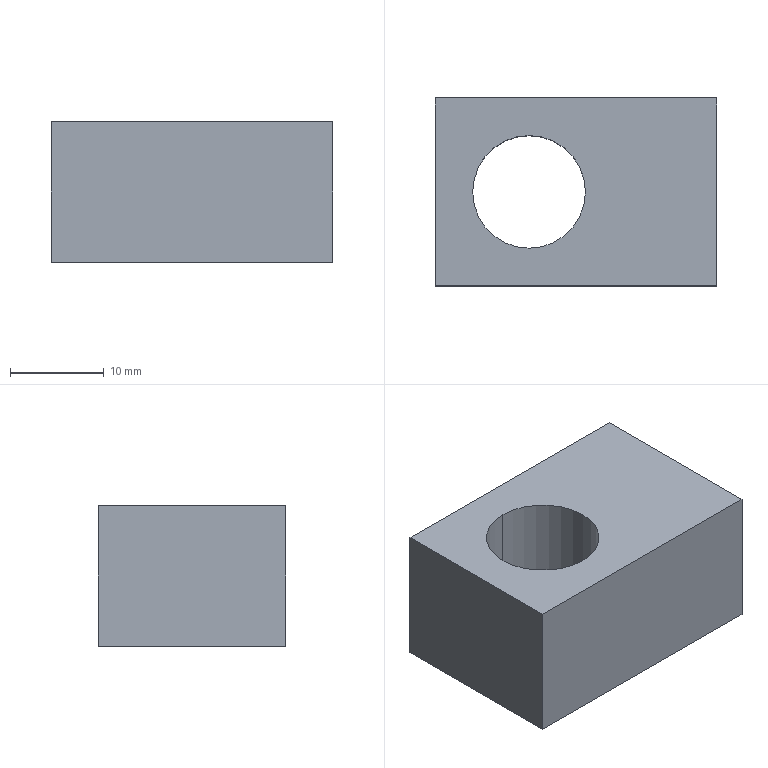Part | STEP file | Positioning_id1962_x_t | 1 solid | 11 faces | box 30 x 20 x 15 mm | volume 7190 mm3 | plane 7 | cylinder 4 | commonest cylinder face diameters 6 x2 12 x2
STEP:
#1=CARTESIAN_POINT('',(0.,0.,0.));
#2=DIRECTION('',(0.,0.,1.));
#3=DIRECTION('',(1.,0.,0.));
#4=AXIS2_PLACEMENT_3D('',#1,#2,#3);
#5=CARTESIAN_POINT('',(-706.002,0.5,354.5));
#6=VERTEX_POINT('',#5);
#7=CARTESIAN_POINT('',(-706.002,-5.5,354.5));
#8=VERTEX_POINT('',#7);
#9=CARTESIAN_POINT('',(-706.002,-2.5,354.5));
#10=DIRECTION('',(-1.,0.,0.));
#11=DIRECTION('',(0.,0.,-1.));
#12=AXIS2_PLACEMENT_3D('',#9,#10,#11);
#13=CIRCLE('',#12,3.);
#14=CARTESIAN_POINT('',(-656.002,-2.5,354.5));
#15=DIRECTION('',(1.,0.,0.));
#16=DIRECTION('',(0.,-1.,0.));
#17=AXIS2_PLACEMENT_3D('',#14,#15,#16);
#18=CYLINDRICAL_SURFACE('',#17,3.);
#19=CARTESIAN_POINT('',(7.854,-50.));
#20=DIRECTION('',(-1.,0.));
#21=VECTOR('',#20,1.);
#22=LINE('',#19,#21);
#23=(GEOMETRIC_REPRESENTATION_CONTEXT(2)PARAMETRIC_REPRESENTATION_CONTEXT()REPRESENTATION_CONTEXT('',''));
#24=DEFINITIONAL_REPRESENTATION('',(#22),#23);
#25=PCURVE('',#18,#24);
#26=CARTESIAN_POINT('',(-706.002,-2.5,354.5));
#27=DIRECTION('',(-1.,0.,0.));
#28=DIRECTION('',(0.,-1.,0.));
#29=AXIS2_PLACEMENT_3D('',#26,#27,#28);
#30=PLANE('',#29);
#31=CARTESIAN_POINT('',(0.,0.));
#32=DIRECTION('',(0.,-1.));
#33=AXIS2_PLACEMENT_2D('',#31,#32);
#34=CIRCLE('',#33,3.);
#35=(GEOMETRIC_REPRESENTATION_CONTEXT(2)PARAMETRIC_REPRESENTATION_CONTEXT()REPRESENTATION_CONTEXT('',''));
#36=DEFINITIONAL_REPRESENTATION('',(#34),#35);
#37=PCURVE('',#30,#36);
#38=SURFACE_CURVE('',#13,(#25,#37),.PCURVE_S1.);
#39=EDGE_CURVE('',#6,#8,#38,.T.);
#40=ORIENTED_EDGE('',*,*,#39,.F.);
#41=CARTESIAN_POINT('',(-702.002,0.5,354.5));
#42=VERTEX_POINT('',#41);
#43=CARTESIAN_POINT('',(-702.002,0.5,354.5));
#44=DIRECTION('',(1.,0.,0.));
#45=VECTOR('',#44,1.);
#46=LINE('',#43,#45);
#47=CARTESIAN_POINT('',(3.142,-46.));
#48=DIRECTION('',(0.,1.));
#49=VECTOR('',#48,1.);
#50=LINE('',#47,#49);
#51=(GEOMETRIC_REPRESENTATION_CONTEXT(2)PARAMETRIC_REPRESENTATION_CONTEXT()REPRESENTATION_CONTEXT('',''));
#52=DEFINITIONAL_REPRESENTATION('',(#50),#51);
#53=PCURVE('',#18,#52);
#54=CARTESIAN_POINT('',(-656.002,-2.5,354.5));
#55=DIRECTION('',(1.,0.,0.));
#56=DIRECTION('',(0.,-1.,0.));
#57=AXIS2_PLACEMENT_3D('',#54,#55,#56);
#58=CYLINDRICAL_SURFACE('',#57,3.);
#59=CARTESIAN_POINT('',(3.142,-46.));
#60=DIRECTION('',(0.,1.));
#61=VECTOR('',#60,1.);
#62=LINE('',#59,#61);
#63=(GEOMETRIC_REPRESENTATION_CONTEXT(2)PARAMETRIC_REPRESENTATION_CONTEXT()REPRESENTATION_CONTEXT('',''));
#64=DEFINITIONAL_REPRESENTATION('',(#62),#63);
#65=PCURVE('',#58,#64);
#66=SURFACE_CURVE('',#46,(#53,#65),.PCURVE_S1.);
#67=EDGE_CURVE('',#6,#42,#66,.T.);
#68=ORIENTED_EDGE('',*,*,#67,.T.);
#69=CARTESIAN_POINT('',(-702.002,-5.5,354.5));
#70=VERTEX_POINT('',#69);
#71=CARTESIAN_POINT('',(-702.002,-2.5,354.5));
#72=DIRECTION('',(1.,0.,0.));
#73=DIRECTION('',(0.,0.,-1.));
#74=AXIS2_PLACEMENT_3D('',#71,#72,#73);
#75=CIRCLE('',#74,3.);
#76=CARTESIAN_POINT('',(-4.712,-46.));
#77=DIRECTION('',(1.,0.));
#78=VECTOR('',#77,1.);
#79=LINE('',#76,#78);
#80=(GEOMETRIC_REPRESENTATION_CONTEXT(2)PARAMETRIC_REPRESENTATION_CONTEXT()REPRESENTATION_CONTEXT('',''));
#81=DEFINITIONAL_REPRESENTATION('',(#79),#80);
#82=PCURVE('',#18,#81);
#83=CARTESIAN_POINT('',(-702.002,12.5,362.));
#84=DIRECTION('',(1.,0.,0.));
#85=DIRECTION('',(0.,-1.,0.));
#86=AXIS2_PLACEMENT_3D('',#83,#84,#85);
#87=PLANE('',#86);
#88=CARTESIAN_POINT('',(15.,7.5));
#89=DIRECTION('',(0.,1.));
#90=AXIS2_PLACEMENT_2D('',#88,#89);
#91=CIRCLE('',#90,3.);
#92=(GEOMETRIC_REPRESENTATION_CONTEXT(2)PARAMETRIC_REPRESENTATION_CONTEXT()REPRESENTATION_CONTEXT('',''));
#93=DEFINITIONAL_REPRESENTATION('',(#91),#92);
#94=PCURVE('',#87,#93);
#95=SURFACE_CURVE('',#75,(#82,#94),.PCURVE_S1.);
#96=EDGE_CURVE('',#70,#42,#95,.T.);
#97=ORIENTED_EDGE('',*,*,#96,.F.);
#98=CARTESIAN_POINT('',(-702.002,-5.5,354.5));
#99=DIRECTION('',(-1.,0.,0.));
#100=VECTOR('',#99,1.);
#101=LINE('',#98,#100);
#102=CARTESIAN_POINT('',(0.,-46.));
#103=DIRECTION('',(0.,-1.));
#104=VECTOR('',#103,1.);
#105=LINE('',#102,#104);
#106=(GEOMETRIC_REPRESENTATION_CONTEXT(2)PARAMETRIC_REPRESENTATION_CONTEXT()REPRESENTATION_CONTEXT('',''));
#107=DEFINITIONAL_REPRESENTATION('',(#105),#106);
#108=PCURVE('',#18,#107);
#109=CARTESIAN_POINT('',(6.283,-46.));
#110=DIRECTION('',(0.,-1.));
#111=VECTOR('',#110,1.);
#112=LINE('',#109,#111);
#113=(GEOMETRIC_REPRESENTATION_CONTEXT(2)PARAMETRIC_REPRESENTATION_CONTEXT()REPRESENTATION_CONTEXT('',''));
#114=DEFINITIONAL_REPRESENTATION('',(#112),#113);
#115=PCURVE('',#58,#114);
#116=SURFACE_CURVE('',#101,(#108,#115),.PCURVE_S1.);
#117=EDGE_CURVE('',#70,#8,#116,.T.);
#118=ORIENTED_EDGE('',*,*,#117,.T.);
#119=EDGE_LOOP('',(#40,#68,#97,#118));
#120=FACE_BOUND('',#119,.F.);
#121=ADVANCED_FACE('',(#120),#18,.F.);
#122=ORIENTED_EDGE('',*,*,#39,.F.);
#123=CARTESIAN_POINT('',(-706.002,-5.5,354.5));
#124=CARTESIAN_POINT('',(-706.002,-5.5,357.5));
#125=CARTESIAN_POINT('',(-706.002,-2.5,359.));
#126=CARTESIAN_POINT('',(-706.002,0.5,357.5));
#127=CARTESIAN_POINT('',(-706.002,0.5,354.5));
#128=(BOUNDED_CURVE()B_SPLINE_CURVE(4,(#123,#124,#125,#126,#127),.UNSPECIFIED.,.F.,.F.)B_SPLINE_CURVE_WITH_KNOTS((5,5),(0.,1.),.PIECEWISE_BEZIER_KNOTS.)CURVE()GEOMETRIC_REPRESENTATION_ITEM()RATIONAL_B_SPLINE_CURVE((1.,0.7071,0.6667,0.7071,1.))REPRESENTATION_ITEM(''));
#129=CARTESIAN_POINT('',(3.,0.));
#130=CARTESIAN_POINT('',(3.,3.));
#131=CARTESIAN_POINT('',(0.,4.5));
#132=CARTESIAN_POINT('',(-3.,3.));
#133=CARTESIAN_POINT('',(-3.,0.));
#134=(BOUNDED_CURVE()B_SPLINE_CURVE(4,(#129,#130,#131,#132,#133),.UNSPECIFIED.,.F.,.F.)B_SPLINE_CURVE_WITH_KNOTS((5,5),(0.,1.),.PIECEWISE_BEZIER_KNOTS.)CURVE()GEOMETRIC_REPRESENTATION_ITEM()RATIONAL_B_SPLINE_CURVE((1.,0.7071,0.6667,0.7071,1.))REPRESENTATION_ITEM(''));
#135=(GEOMETRIC_REPRESENTATION_CONTEXT(2)PARAMETRIC_REPRESENTATION_CONTEXT()REPRESENTATION_CONTEXT('',''));
#136=DEFINITIONAL_REPRESENTATION('',(#134),#135);
#137=PCURVE('',#30,#136);
#138=CARTESIAN_POINT('',(6.283,-50.));
#139=CARTESIAN_POINT('',(6.24,-50.));
#140=CARTESIAN_POINT('',(6.153,-50.));
#141=CARTESIAN_POINT('',(6.02,-50.));
#142=CARTESIAN_POINT('',(5.883,-50.));
#143=CARTESIAN_POINT('',(5.744,-50.));
#144=CARTESIAN_POINT('',(5.602,-50.));
#145=CARTESIAN_POINT('',(5.457,-50.));
#146=CARTESIAN_POINT('',(5.311,-50.));
#147=CARTESIAN_POINT('',(5.163,-50.));
#148=CARTESIAN_POINT('',(5.013,-50.));
#149=CARTESIAN_POINT('',(4.863,-50.));
#150=CARTESIAN_POINT('',(4.712,-50.));
#151=CARTESIAN_POINT('',(4.562,-50.));
#152=CARTESIAN_POINT('',(4.412,-50.));
#153=CARTESIAN_POINT('',(4.262,-50.));
#154=CARTESIAN_POINT('',(4.114,-50.));
#155=CARTESIAN_POINT('',(3.968,-50.));
#156=CARTESIAN_POINT('',(3.823,-50.));
#157=CARTESIAN_POINT('',(3.681,-50.));
#158=CARTESIAN_POINT('',(3.542,-50.));
#159=CARTESIAN_POINT('',(3.405,-50.));
#160=CARTESIAN_POINT('',(3.271,-50.));
#161=CARTESIAN_POINT('',(3.184,-50.));
#162=CARTESIAN_POINT('',(3.142,-50.));
#163=B_SPLINE_CURVE_WITH_KNOTS('',3,(#138,#139,#140,#141,#142,#143,#144,#145,#146,#147,#148,#149,#150,#151,#152,#153,#154,#155,#156,#157,#158,#159,#160,#161,#162),.UNSPECIFIED.,.F.,.F.,(4,1,1,1,1,1,1,1,1,1,1,1,1,1,1,1,1,1,1,1,1,1,4),(0.,0.04545,0.09091,0.1364,0.1818,0.2273,0.2727,0.3182,0.3636,0.4091,0.4545,0.5,0.5455,0.5909,0.6364,0.6818,0.7273,0.7727,0.8182,0.8636,0.9091,0.9545,1.),.QUASI_UNIFORM_KNOTS.);
#164=(GEOMETRIC_REPRESENTATION_CONTEXT(2)PARAMETRIC_REPRESENTATION_CONTEXT()REPRESENTATION_CONTEXT('',''));
#165=DEFINITIONAL_REPRESENTATION('',(#163),#164);
#166=PCURVE('',#58,#165);
#167=SURFACE_CURVE('',#128,(#137,#166),.PCURVE_S1.);
#168=EDGE_CURVE('',#8,#6,#167,.T.);
#169=ORIENTED_EDGE('',*,*,#168,.F.);
#170=EDGE_LOOP('',(#122,#169));
#171=FACE_BOUND('',#170,.T.);
#172=ADVANCED_FACE('',(#171),#30,.F.);
#173=CARTESIAN_POINT('',(-702.002,-10.,362.));
#174=VERTEX_POINT('',#173);
#175=CARTESIAN_POINT('',(-732.002,-10.,362.));
#176=VERTEX_POINT('',#175);
#177=CARTESIAN_POINT('',(-702.002,-10.,362.));
#178=DIRECTION('',(-1.,0.,0.));
#179=VECTOR('',#178,1.);
#180=LINE('',#177,#179);
#181=CARTESIAN_POINT('',(-656.002,-10.,364.5));
#182=DIRECTION('',(0.,-1.,0.));
#183=DIRECTION('',(0.,0.,1.));
#184=AXIS2_PLACEMENT_3D('',#181,#182,#183);
#185=PLANE('',#184);
#186=CARTESIAN_POINT('',(-2.5,46.));
#187=DIRECTION('',(0.,1.));
#188=VECTOR('',#187,1.);
#189=LINE('',#186,#188);
#190=(GEOMETRIC_REPRESENTATION_CONTEXT(2)PARAMETRIC_REPRESENTATION_CONTEXT()REPRESENTATION_CONTEXT('',''));
#191=DEFINITIONAL_REPRESENTATION('',(#189),#190);
#192=PCURVE('',#185,#191);
#193=CARTESIAN_POINT('',(-714.502,-6.25,362.));
#194=DIRECTION('',(0.,0.,1.));
#195=DIRECTION('',(1.,0.,0.));
#196=AXIS2_PLACEMENT_3D('',#193,#194,#195);
#197=PLANE('',#196);
#198=CARTESIAN_POINT('',(12.5,-3.75));
#199=DIRECTION('',(-1.,0.));
#200=VECTOR('',#199,1.);
#201=LINE('',#198,#200);
#202=(GEOMETRIC_REPRESENTATION_CONTEXT(2)PARAMETRIC_REPRESENTATION_CONTEXT()REPRESENTATION_CONTEXT('',''));
#203=DEFINITIONAL_REPRESENTATION('',(#201),#202);
#204=PCURVE('',#197,#203);
#205=SURFACE_CURVE('',#180,(#192,#204),.PCURVE_S1.);
#206=EDGE_CURVE('',#174,#176,#205,.T.);
#207=ORIENTED_EDGE('',*,*,#206,.T.);
#208=CARTESIAN_POINT('',(-732.002,-10.,347.));
#209=VERTEX_POINT('',#208);
#210=CARTESIAN_POINT('',(-732.002,-10.,362.));
#211=DIRECTION('',(0.,0.,-1.));
#212=VECTOR('',#211,1.);
#213=LINE('',#210,#212);
#214=CARTESIAN_POINT('',(-2.5,76.));
#215=DIRECTION('',(-1.,0.));
#216=VECTOR('',#215,1.);
#217=LINE('',#214,#216);
#218=(GEOMETRIC_REPRESENTATION_CONTEXT(2)PARAMETRIC_REPRESENTATION_CONTEXT()REPRESENTATION_CONTEXT('',''));
#219=DEFINITIONAL_REPRESENTATION('',(#217),#218);
#220=PCURVE('',#185,#219);
#221=CARTESIAN_POINT('',(-732.002,-6.25,354.5));
#222=DIRECTION('',(-1.,0.,0.));
#223=DIRECTION('',(0.,0.,1.));
#224=AXIS2_PLACEMENT_3D('',#221,#222,#223);
#225=PLANE('',#224);
#226=CARTESIAN_POINT('',(7.5,-3.75));
#227=DIRECTION('',(-1.,0.));
#228=VECTOR('',#227,1.);
#229=LINE('',#226,#228);
#230=(GEOMETRIC_REPRESENTATION_CONTEXT(2)PARAMETRIC_REPRESENTATION_CONTEXT()REPRESENTATION_CONTEXT('',''));
#231=DEFINITIONAL_REPRESENTATION('',(#229),#230);
#232=PCURVE('',#225,#231);
#233=SURFACE_CURVE('',#213,(#220,#232),.PCURVE_S1.);
#234=EDGE_CURVE('',#176,#209,#233,.T.);
#235=ORIENTED_EDGE('',*,*,#234,.T.);
#236=CARTESIAN_POINT('',(-702.002,-10.,347.));
#237=VERTEX_POINT('',#236);
#238=CARTESIAN_POINT('',(-732.002,-10.,347.));
#239=DIRECTION('',(1.,0.,0.));
#240=VECTOR('',#239,1.);
#241=LINE('',#238,#240);
#242=CARTESIAN_POINT('',(-17.5,76.));
#243=DIRECTION('',(0.,-1.));
#244=VECTOR('',#243,1.);
#245=LINE('',#242,#244);
#246=(GEOMETRIC_REPRESENTATION_CONTEXT(2)PARAMETRIC_REPRESENTATION_CONTEXT()REPRESENTATION_CONTEXT('',''));
#247=DEFINITIONAL_REPRESENTATION('',(#245),#246);
#248=PCURVE('',#185,#247);
#249=CARTESIAN_POINT('',(-714.502,-6.25,347.));
#250=DIRECTION('',(0.,0.,-1.));
#251=DIRECTION('',(-1.,0.,0.));
#252=AXIS2_PLACEMENT_3D('',#249,#250,#251);
#253=PLANE('',#252);
#254=CARTESIAN_POINT('',(17.5,-3.75));
#255=DIRECTION('',(-1.,0.));
#256=VECTOR('',#255,1.);
#257=LINE('',#254,#256);
#258=(GEOMETRIC_REPRESENTATION_CONTEXT(2)PARAMETRIC_REPRESENTATION_CONTEXT()REPRESENTATION_CONTEXT('',''));
#259=DEFINITIONAL_REPRESENTATION('',(#257),#258);
#260=PCURVE('',#253,#259);
#261=SURFACE_CURVE('',#241,(#248,#260),.PCURVE_S1.);
#262=EDGE_CURVE('',#209,#237,#261,.T.);
#263=ORIENTED_EDGE('',*,*,#262,.T.);
#264=CARTESIAN_POINT('',(-702.002,-10.,362.));
#265=DIRECTION('',(0.,0.,-1.));
#266=VECTOR('',#265,1.);
#267=LINE('',#264,#266);
#268=CARTESIAN_POINT('',(-2.5,46.));
#269=DIRECTION('',(-1.,0.));
#270=VECTOR('',#269,1.);
#271=LINE('',#268,#270);
#272=(GEOMETRIC_REPRESENTATION_CONTEXT(2)PARAMETRIC_REPRESENTATION_CONTEXT()REPRESENTATION_CONTEXT('',''));
#273=DEFINITIONAL_REPRESENTATION('',(#271),#272);
#274=PCURVE('',#185,#273);
#275=CARTESIAN_POINT('',(22.5,0.));
#276=DIRECTION('',(0.,1.));
#277=VECTOR('',#276,1.);
#278=LINE('',#275,#277);
#279=(GEOMETRIC_REPRESENTATION_CONTEXT(2)PARAMETRIC_REPRESENTATION_CONTEXT()REPRESENTATION_CONTEXT('',''));
#280=DEFINITIONAL_REPRESENTATION('',(#278),#279);
#281=PCURVE('',#87,#280);
#282=SURFACE_CURVE('',#267,(#274,#281),.PCURVE_S1.);
#283=EDGE_CURVE('',#174,#237,#282,.T.);
#284=ORIENTED_EDGE('',*,*,#283,.F.);
#285=EDGE_LOOP('',(#207,#235,#263,#284));
#286=FACE_BOUND('',#285,.T.);
#287=ADVANCED_FACE('',(#286),#185,.T.);
#288=CARTESIAN_POINT('',(-722.002,-6.,347.));
#289=VERTEX_POINT('',#288);
#290=CARTESIAN_POINT('',(-722.002,6.,347.));
#291=VERTEX_POINT('',#290);
#292=CARTESIAN_POINT('',(-722.002,-0.00002593,347.));
#293=DIRECTION('',(0.,0.,-1.));
#294=DIRECTION('',(0.,-1.,0.));
#295=AXIS2_PLACEMENT_3D('',#292,#293,#294);
#296=CIRCLE('',#295,6.);
#297=CARTESIAN_POINT('',(7.5,6.25));
#298=DIRECTION('',(0.,-1.));
#299=AXIS2_PLACEMENT_2D('',#297,#298);
#300=CIRCLE('',#299,6.);
#301=(GEOMETRIC_REPRESENTATION_CONTEXT(2)PARAMETRIC_REPRESENTATION_CONTEXT()REPRESENTATION_CONTEXT('',''));
#302=DEFINITIONAL_REPRESENTATION('',(#300),#301);
#303=PCURVE('',#253,#302);
#304=CARTESIAN_POINT('',(-722.002,-0.00002593,342.));
#305=DIRECTION('',(0.,0.,-1.));
#306=DIRECTION('',(0.,1.,0.));
#307=AXIS2_PLACEMENT_3D('',#304,#305,#306);
#308=CYLINDRICAL_SURFACE('',#307,6.);
#309=CARTESIAN_POINT('',(3.142,-5.));
#310=DIRECTION('',(1.,0.));
#311=VECTOR('',#310,1.);
#312=LINE('',#309,#311);
#313=(GEOMETRIC_REPRESENTATION_CONTEXT(2)PARAMETRIC_REPRESENTATION_CONTEXT()REPRESENTATION_CONTEXT('',''));
#314=DEFINITIONAL_REPRESENTATION('',(#312),#313);
#315=PCURVE('',#308,#314);
#316=SURFACE_CURVE('',#296,(#303,#315),.PCURVE_S1.);
#317=EDGE_CURVE('',#289,#291,#316,.T.);
#318=ORIENTED_EDGE('',*,*,#317,.F.);
#319=CARTESIAN_POINT('',(-722.002,-0.00002593,347.));
#320=DIRECTION('',(0.,0.,-1.));
#321=DIRECTION('',(0.,1.,0.));
#322=AXIS2_PLACEMENT_3D('',#319,#320,#321);
#323=CIRCLE('',#322,6.);
#324=CARTESIAN_POINT('',(7.5,6.25));
#325=DIRECTION('',(0.,1.));
#326=AXIS2_PLACEMENT_2D('',#324,#325);
#327=CIRCLE('',#326,6.);
#328=(GEOMETRIC_REPRESENTATION_CONTEXT(2)PARAMETRIC_REPRESENTATION_CONTEXT()REPRESENTATION_CONTEXT('',''));
#329=DEFINITIONAL_REPRESENTATION('',(#327),#328);
#330=PCURVE('',#253,#329);
#331=CARTESIAN_POINT('',(-722.002,-0.00002593,342.));
#332=DIRECTION('',(0.,0.,-1.));
#333=DIRECTION('',(0.,1.,0.));
#334=AXIS2_PLACEMENT_3D('',#331,#332,#333);
#335=CYLINDRICAL_SURFACE('',#334,6.);
#336=CARTESIAN_POINT('',(0.,-5.));
#337=DIRECTION('',(1.,0.));
#338=VECTOR('',#337,1.);
#339=LINE('',#336,#338);
#340=(GEOMETRIC_REPRESENTATION_CONTEXT(2)PARAMETRIC_REPRESENTATION_CONTEXT()REPRESENTATION_CONTEXT('',''));
#341=DEFINITIONAL_REPRESENTATION('',(#339),#340);
#342=PCURVE('',#335,#341);
#343=SURFACE_CURVE('',#323,(#330,#342),.PCURVE_S1.);
#344=EDGE_CURVE('',#291,#289,#343,.T.);
#345=ORIENTED_EDGE('',*,*,#344,.F.);
#346=EDGE_LOOP('',(#318,#345));
#347=FACE_BOUND('',#346,.T.);
#348=CARTESIAN_POINT('',(-702.002,10.,347.));
#349=VERTEX_POINT('',#348);
#350=CARTESIAN_POINT('',(-732.002,10.,347.));
#351=VERTEX_POINT('',#350);
#352=CARTESIAN_POINT('',(-702.002,10.,347.));
#353=DIRECTION('',(-1.,0.,0.));
#354=VECTOR('',#353,1.);
#355=LINE('',#352,#354);
#356=CARTESIAN_POINT('',(-12.5,16.25));
#357=DIRECTION('',(1.,0.));
#358=VECTOR('',#357,1.);
#359=LINE('',#356,#358);
#360=(GEOMETRIC_REPRESENTATION_CONTEXT(2)PARAMETRIC_REPRESENTATION_CONTEXT()REPRESENTATION_CONTEXT('',''));
#361=DEFINITIONAL_REPRESENTATION('',(#359),#360);
#362=PCURVE('',#253,#361);
#363=CARTESIAN_POINT('',(-714.502,10.,354.5));
#364=DIRECTION('',(0.,1.,0.));
#365=DIRECTION('',(0.,0.,-1.));
#366=AXIS2_PLACEMENT_3D('',#363,#364,#365);
#367=PLANE('',#366);
#368=CARTESIAN_POINT('',(7.5,-12.5));
#369=DIRECTION('',(0.,1.));
#370=VECTOR('',#369,1.);
#371=LINE('',#368,#370);
#372=(GEOMETRIC_REPRESENTATION_CONTEXT(2)PARAMETRIC_REPRESENTATION_CONTEXT()REPRESENTATION_CONTEXT('',''));
#373=DEFINITIONAL_REPRESENTATION('',(#371),#372);
#374=PCURVE('',#367,#373);
#375=SURFACE_CURVE('',#355,(#362,#374),.PCURVE_S1.);
#376=EDGE_CURVE('',#349,#351,#375,.T.);
#377=ORIENTED_EDGE('',*,*,#376,.F.);
#378=CARTESIAN_POINT('',(-702.002,-10.,347.));
#379=DIRECTION('',(0.,1.,0.));
#380=VECTOR('',#379,1.);
#381=LINE('',#378,#380);
#382=CARTESIAN_POINT('',(-12.5,-3.75));
#383=DIRECTION('',(0.,1.));
#384=VECTOR('',#383,1.);
#385=LINE('',#382,#384);
#386=(GEOMETRIC_REPRESENTATION_CONTEXT(2)PARAMETRIC_REPRESENTATION_CONTEXT()REPRESENTATION_CONTEXT('',''));
#387=DEFINITIONAL_REPRESENTATION('',(#385),#386);
#388=PCURVE('',#253,#387);
#389=CARTESIAN_POINT('',(22.5,15.));
#390=DIRECTION('',(-1.,0.));
#391=VECTOR('',#390,1.);
#392=LINE('',#389,#391);
#393=(GEOMETRIC_REPRESENTATION_CONTEXT(2)PARAMETRIC_REPRESENTATION_CONTEXT()REPRESENTATION_CONTEXT('',''));
#394=DEFINITIONAL_REPRESENTATION('',(#392),#393);
#395=PCURVE('',#87,#394);
#396=SURFACE_CURVE('',#381,(#388,#395),.PCURVE_S1.);
#397=EDGE_CURVE('',#237,#349,#396,.T.);
#398=ORIENTED_EDGE('',*,*,#397,.F.);
#399=ORIENTED_EDGE('',*,*,#262,.F.);
#400=CARTESIAN_POINT('',(-732.002,10.,347.));
#401=DIRECTION('',(0.,-1.,0.));
#402=VECTOR('',#401,1.);
#403=LINE('',#400,#402);
#404=CARTESIAN_POINT('',(17.5,16.25));
#405=DIRECTION('',(0.,-1.));
#406=VECTOR('',#405,1.);
#407=LINE('',#404,#406);
#408=(GEOMETRIC_REPRESENTATION_CONTEXT(2)PARAMETRIC_REPRESENTATION_CONTEXT()REPRESENTATION_CONTEXT('',''));
#409=DEFINITIONAL_REPRESENTATION('',(#407),#408);
#410=PCURVE('',#253,#409);
#411=CARTESIAN_POINT('',(-7.5,16.25));
#412=DIRECTION('',(0.,-1.));
#413=VECTOR('',#412,1.);
#414=LINE('',#411,#413);
#415=(GEOMETRIC_REPRESENTATION_CONTEXT(2)PARAMETRIC_REPRESENTATION_CONTEXT()REPRESENTATION_CONTEXT('',''));
#416=DEFINITIONAL_REPRESENTATION('',(#414),#415);
#417=PCURVE('',#225,#416);
#418=SURFACE_CURVE('',#403,(#410,#417),.PCURVE_S1.);
#419=EDGE_CURVE('',#351,#209,#418,.T.);
#420=ORIENTED_EDGE('',*,*,#419,.F.);
#421=EDGE_LOOP('',(#377,#398,#399,#420));
#422=FACE_BOUND('',#421,.T.);
#423=ADVANCED_FACE('',(#347,#422),#253,.T.);
#424=CARTESIAN_POINT('',(-702.002,10.,362.));
#425=VERTEX_POINT('',#424);
#426=CARTESIAN_POINT('',(-702.002,10.,362.));
#427=DIRECTION('',(0.,0.,-1.));
#428=VECTOR('',#427,1.);
#429=LINE('',#426,#428);
#430=CARTESIAN_POINT('',(-7.5,-12.5));
#431=DIRECTION('',(1.,0.));
#432=VECTOR('',#431,1.);
#433=LINE('',#430,#432);
#434=(GEOMETRIC_REPRESENTATION_CONTEXT(2)PARAMETRIC_REPRESENTATION_CONTEXT()REPRESENTATION_CONTEXT('',''));
#435=DEFINITIONAL_REPRESENTATION('',(#433),#434);
#436=PCURVE('',#367,#435);
#437=CARTESIAN_POINT('',(2.5,0.));
#438=DIRECTION('',(0.,1.));
#439=VECTOR('',#438,1.);
#440=LINE('',#437,#439);
#441=(GEOMETRIC_REPRESENTATION_CONTEXT(2)PARAMETRIC_REPRESENTATION_CONTEXT()REPRESENTATION_CONTEXT('',''));
#442=DEFINITIONAL_REPRESENTATION('',(#440),#441);
#443=PCURVE('',#87,#442);
#444=SURFACE_CURVE('',#429,(#436,#443),.PCURVE_S1.);
#445=EDGE_CURVE('',#425,#349,#444,.T.);
#446=ORIENTED_EDGE('',*,*,#445,.T.);
#447=ORIENTED_EDGE('',*,*,#376,.T.);
#448=CARTESIAN_POINT('',(-732.002,10.,362.));
#449=VERTEX_POINT('',#448);
#450=CARTESIAN_POINT('',(-732.002,10.,362.));
#451=DIRECTION('',(0.,0.,-1.));
#452=VECTOR('',#451,1.);
#453=LINE('',#450,#452);
#454=CARTESIAN_POINT('',(-7.5,17.5));
#455=DIRECTION('',(1.,0.));
#456=VECTOR('',#455,1.);
#457=LINE('',#454,#456);
#458=(GEOMETRIC_REPRESENTATION_CONTEXT(2)PARAMETRIC_REPRESENTATION_CONTEXT()REPRESENTATION_CONTEXT('',''));
#459=DEFINITIONAL_REPRESENTATION('',(#457),#458);
#460=PCURVE('',#367,#459);
#461=CARTESIAN_POINT('',(7.5,16.25));
#462=DIRECTION('',(-1.,0.));
#463=VECTOR('',#462,1.);
#464=LINE('',#461,#463);
#465=(GEOMETRIC_REPRESENTATION_CONTEXT(2)PARAMETRIC_REPRESENTATION_CONTEXT()REPRESENTATION_CONTEXT('',''));
#466=DEFINITIONAL_REPRESENTATION('',(#464),#465);
#467=PCURVE('',#225,#466);
#468=SURFACE_CURVE('',#453,(#460,#467),.PCURVE_S1.);
#469=EDGE_CURVE('',#449,#351,#468,.T.);
#470=ORIENTED_EDGE('',*,*,#469,.F.);
#471=CARTESIAN_POINT('',(-732.002,10.,362.));
#472=DIRECTION('',(1.,0.,0.));
#473=VECTOR('',#472,1.);
#474=LINE('',#471,#473);
#475=CARTESIAN_POINT('',(-7.5,17.5));
#476=DIRECTION('',(0.,-1.));
#477=VECTOR('',#476,1.);
#478=LINE('',#475,#477);
#479=(GEOMETRIC_REPRESENTATION_CONTEXT(2)PARAMETRIC_REPRESENTATION_CONTEXT()REPRESENTATION_CONTEXT('',''));
#480=DEFINITIONAL_REPRESENTATION('',(#478),#479);
#481=PCURVE('',#367,#480);
#482=CARTESIAN_POINT('',(-17.5,16.25));
#483=DIRECTION('',(1.,0.));
#484=VECTOR('',#483,1.);
#485=LINE('',#482,#484);
#486=(GEOMETRIC_REPRESENTATION_CONTEXT(2)PARAMETRIC_REPRESENTATION_CONTEXT()REPRESENTATION_CONTEXT('',''));
#487=DEFINITIONAL_REPRESENTATION('',(#485),#486);
#488=PCURVE('',#197,#487);
#489=SURFACE_CURVE('',#474,(#481,#488),.PCURVE_S1.);
#490=EDGE_CURVE('',#449,#425,#489,.T.);
#491=ORIENTED_EDGE('',*,*,#490,.T.);
#492=EDGE_LOOP('',(#446,#447,#470,#491));
#493=FACE_BOUND('',#492,.T.);
#494=ADVANCED_FACE('',(#493),#367,.T.);
#495=CARTESIAN_POINT('',(-722.002,-6.,362.));
#496=VERTEX_POINT('',#495);
#497=CARTESIAN_POINT('',(-722.002,6.,362.));
#498=VERTEX_POINT('',#497);
#499=CARTESIAN_POINT('',(-722.002,-0.00002593,362.));
#500=DIRECTION('',(0.,0.,1.));
#501=DIRECTION('',(0.,-1.,0.));
#502=AXIS2_PLACEMENT_3D('',#499,#500,#501);
#503=CIRCLE('',#502,6.);
#504=CARTESIAN_POINT('',(-7.5,6.25));
#505=DIRECTION('',(0.,-1.));
#506=AXIS2_PLACEMENT_2D('',#504,#505);
#507=CIRCLE('',#506,6.);
#508=(GEOMETRIC_REPRESENTATION_CONTEXT(2)PARAMETRIC_REPRESENTATION_CONTEXT()REPRESENTATION_CONTEXT('',''));
#509=DEFINITIONAL_REPRESENTATION('',(#507),#508);
#510=PCURVE('',#197,#509);
#511=CARTESIAN_POINT('',(3.142,-20.));
#512=DIRECTION('',(-1.,0.));
#513=VECTOR('',#512,1.);
#514=LINE('',#511,#513);
#515=(GEOMETRIC_REPRESENTATION_CONTEXT(2)PARAMETRIC_REPRESENTATION_CONTEXT()REPRESENTATION_CONTEXT('',''));
#516=DEFINITIONAL_REPRESENTATION('',(#514),#515);
#517=PCURVE('',#335,#516);
#518=SURFACE_CURVE('',#503,(#510,#517),.PCURVE_S1.);
#519=EDGE_CURVE('',#496,#498,#518,.T.);
#520=ORIENTED_EDGE('',*,*,#519,.F.);
#521=CARTESIAN_POINT('',(-722.002,-0.00002593,362.));
#522=DIRECTION('',(0.,0.,1.));
#523=DIRECTION('',(0.,1.,0.));
#524=AXIS2_PLACEMENT_3D('',#521,#522,#523);
#525=CIRCLE('',#524,6.);
#526=CARTESIAN_POINT('',(-7.5,6.25));
#527=DIRECTION('',(0.,1.));
#528=AXIS2_PLACEMENT_2D('',#526,#527);
#529=CIRCLE('',#528,6.);
#530=(GEOMETRIC_REPRESENTATION_CONTEXT(2)PARAMETRIC_REPRESENTATION_CONTEXT()REPRESENTATION_CONTEXT('',''));
#531=DEFINITIONAL_REPRESENTATION('',(#529),#530);
#532=PCURVE('',#197,#531);
#533=CARTESIAN_POINT('',(6.283,-20.));
#534=DIRECTION('',(-1.,0.));
#535=VECTOR('',#534,1.);
#536=LINE('',#533,#535);
#537=(GEOMETRIC_REPRESENTATION_CONTEXT(2)PARAMETRIC_REPRESENTATION_CONTEXT()REPRESENTATION_CONTEXT('',''));
#538=DEFINITIONAL_REPRESENTATION('',(#536),#537);
#539=PCURVE('',#308,#538);
#540=SURFACE_CURVE('',#525,(#532,#539),.PCURVE_S1.);
#541=EDGE_CURVE('',#498,#496,#540,.T.);
#542=ORIENTED_EDGE('',*,*,#541,.F.);
#543=EDGE_LOOP('',(#520,#542));
#544=FACE_BOUND('',#543,.T.);
#545=CARTESIAN_POINT('',(-702.002,10.,362.));
#546=DIRECTION('',(0.,-1.,0.));
#547=VECTOR('',#546,1.);
#548=LINE('',#545,#547);
#549=CARTESIAN_POINT('',(12.5,16.25));
#550=DIRECTION('',(0.,-1.));
#551=VECTOR('',#550,1.);
#552=LINE('',#549,#551);
#553=(GEOMETRIC_REPRESENTATION_CONTEXT(2)PARAMETRIC_REPRESENTATION_CONTEXT()REPRESENTATION_CONTEXT('',''));
#554=DEFINITIONAL_REPRESENTATION('',(#552),#553);
#555=PCURVE('',#197,#554);
#556=CARTESIAN_POINT('',(2.5,0.));
#557=DIRECTION('',(1.,0.));
#558=VECTOR('',#557,1.);
#559=LINE('',#556,#558);
#560=(GEOMETRIC_REPRESENTATION_CONTEXT(2)PARAMETRIC_REPRESENTATION_CONTEXT()REPRESENTATION_CONTEXT('',''));
#561=DEFINITIONAL_REPRESENTATION('',(#559),#560);
#562=PCURVE('',#87,#561);
#563=SURFACE_CURVE('',#548,(#555,#562),.PCURVE_S1.);
#564=EDGE_CURVE('',#425,#174,#563,.T.);
#565=ORIENTED_EDGE('',*,*,#564,.F.);
#566=ORIENTED_EDGE('',*,*,#490,.F.);
#567=CARTESIAN_POINT('',(-732.002,-10.,362.));
#568=DIRECTION('',(0.,1.,0.));
#569=VECTOR('',#568,1.);
#570=LINE('',#567,#569);
#571=CARTESIAN_POINT('',(-17.5,-3.75));
#572=DIRECTION('',(0.,1.));
#573=VECTOR('',#572,1.);
#574=LINE('',#571,#573);
#575=(GEOMETRIC_REPRESENTATION_CONTEXT(2)PARAMETRIC_REPRESENTATION_CONTEXT()REPRESENTATION_CONTEXT('',''));
#576=DEFINITIONAL_REPRESENTATION('',(#574),#575);
#577=PCURVE('',#197,#576);
#578=CARTESIAN_POINT('',(7.5,-3.75));
#579=DIRECTION('',(0.,1.));
#580=VECTOR('',#579,1.);
#581=LINE('',#578,#580);
#582=(GEOMETRIC_REPRESENTATION_CONTEXT(2)PARAMETRIC_REPRESENTATION_CONTEXT()REPRESENTATION_CONTEXT('',''));
#583=DEFINITIONAL_REPRESENTATION('',(#581),#582);
#584=PCURVE('',#225,#583);
#585=SURFACE_CURVE('',#570,(#577,#584),.PCURVE_S1.);
#586=EDGE_CURVE('',#176,#449,#585,.T.);
#587=ORIENTED_EDGE('',*,*,#586,.F.);
#588=ORIENTED_EDGE('',*,*,#206,.F.);
#589=EDGE_LOOP('',(#565,#566,#587,#588));
#590=FACE_BOUND('',#589,.T.);
#591=ADVANCED_FACE('',(#544,#590),#197,.T.);
#592=ORIENTED_EDGE('',*,*,#519,.F.);
#593=CARTESIAN_POINT('',(-722.002,-6.,347.));
#594=DIRECTION('',(0.,0.,-1.));
#595=VECTOR('',#594,1.);
#596=LINE('',#593,#595);
#597=CARTESIAN_POINT('',(3.142,-5.));
#598=DIRECTION('',(0.,1.));
#599=VECTOR('',#598,1.);
#600=LINE('',#597,#599);
#601=(GEOMETRIC_REPRESENTATION_CONTEXT(2)PARAMETRIC_REPRESENTATION_CONTEXT()REPRESENTATION_CONTEXT('',''));
#602=DEFINITIONAL_REPRESENTATION('',(#600),#601);
#603=PCURVE('',#335,#602);
#604=CARTESIAN_POINT('',(3.142,-5.));
#605=DIRECTION('',(0.,1.));
#606=VECTOR('',#605,1.);
#607=LINE('',#604,#606);
#608=(GEOMETRIC_REPRESENTATION_CONTEXT(2)PARAMETRIC_REPRESENTATION_CONTEXT()REPRESENTATION_CONTEXT('',''));
#609=DEFINITIONAL_REPRESENTATION('',(#607),#608);
#610=PCURVE('',#308,#609);
#611=SURFACE_CURVE('',#596,(#603,#610),.PCURVE_S1.);
#612=EDGE_CURVE('',#496,#289,#611,.T.);
#613=ORIENTED_EDGE('',*,*,#612,.T.);
#614=ORIENTED_EDGE('',*,*,#344,.F.);
#615=CARTESIAN_POINT('',(-722.002,6.,347.));
#616=DIRECTION('',(0.,0.,1.));
#617=VECTOR('',#616,1.);
#618=LINE('',#615,#617);
#619=CARTESIAN_POINT('',(0.,-5.));
#620=DIRECTION('',(0.,-1.));
#621=VECTOR('',#620,1.);
#622=LINE('',#619,#621);
#623=(GEOMETRIC_REPRESENTATION_CONTEXT(2)PARAMETRIC_REPRESENTATION_CONTEXT()REPRESENTATION_CONTEXT('',''));
#624=DEFINITIONAL_REPRESENTATION('',(#622),#623);
#625=PCURVE('',#335,#624);
#626=CARTESIAN_POINT('',(6.283,-5.));
#627=DIRECTION('',(0.,-1.));
#628=VECTOR('',#627,1.);
#629=LINE('',#626,#628);
#630=(GEOMETRIC_REPRESENTATION_CONTEXT(2)PARAMETRIC_REPRESENTATION_CONTEXT()REPRESENTATION_CONTEXT('',''));
#631=DEFINITIONAL_REPRESENTATION('',(#629),#630);
#632=PCURVE('',#308,#631);
#633=SURFACE_CURVE('',#618,(#625,#632),.PCURVE_S1.);
#634=EDGE_CURVE('',#291,#498,#633,.T.);
#635=ORIENTED_EDGE('',*,*,#634,.T.);
#636=EDGE_LOOP('',(#592,#613,#614,#635));
#637=FACE_BOUND('',#636,.F.);
#638=ADVANCED_FACE('',(#637),#335,.F.);
#639=ORIENTED_EDGE('',*,*,#469,.T.);
#640=ORIENTED_EDGE('',*,*,#419,.T.);
#641=ORIENTED_EDGE('',*,*,#234,.F.);
#642=ORIENTED_EDGE('',*,*,#586,.T.);
#643=EDGE_LOOP('',(#639,#640,#641,#642));
#644=FACE_BOUND('',#643,.T.);
#645=ADVANCED_FACE('',(#644),#225,.T.);
#646=CARTESIAN_POINT('',(-702.002,0.5,354.5));
#647=CARTESIAN_POINT('',(-702.002,0.5,357.5));
#648=CARTESIAN_POINT('',(-702.002,-2.5,359.));
#649=CARTESIAN_POINT('',(-702.002,-5.5,357.5));
#650=CARTESIAN_POINT('',(-702.002,-5.5,354.5));
#651=(BOUNDED_CURVE()B_SPLINE_CURVE(4,(#646,#647,#648,#649,#650),.UNSPECIFIED.,.F.,.F.)B_SPLINE_CURVE_WITH_KNOTS((5,5),(0.,1.),.PIECEWISE_BEZIER_KNOTS.)CURVE()GEOMETRIC_REPRESENTATION_ITEM()RATIONAL_B_SPLINE_CURVE((1.,0.7071,0.6667,0.7071,1.))REPRESENTATION_ITEM(''));
#652=CARTESIAN_POINT('',(12.,7.5));
#653=CARTESIAN_POINT('',(12.,4.5));
#654=CARTESIAN_POINT('',(15.,3.));
#655=CARTESIAN_POINT('',(18.,4.5));
#656=CARTESIAN_POINT('',(18.,7.5));
#657=(BOUNDED_CURVE()B_SPLINE_CURVE(4,(#652,#653,#654,#655,#656),.UNSPECIFIED.,.F.,.F.)B_SPLINE_CURVE_WITH_KNOTS((5,5),(0.,1.),.PIECEWISE_BEZIER_KNOTS.)CURVE()GEOMETRIC_REPRESENTATION_ITEM()RATIONAL_B_SPLINE_CURVE((1.,0.7071,0.6667,0.7071,1.))REPRESENTATION_ITEM(''));
#658=(GEOMETRIC_REPRESENTATION_CONTEXT(2)PARAMETRIC_REPRESENTATION_CONTEXT()REPRESENTATION_CONTEXT('',''));
#659=DEFINITIONAL_REPRESENTATION('',(#657),#658);
#660=PCURVE('',#87,#659);
#661=CARTESIAN_POINT('',(3.142,-46.));
#662=CARTESIAN_POINT('',(3.184,-46.));
#663=CARTESIAN_POINT('',(3.271,-46.));
#664=CARTESIAN_POINT('',(3.405,-46.));
#665=CARTESIAN_POINT('',(3.542,-46.));
#666=CARTESIAN_POINT('',(3.681,-46.));
#667=CARTESIAN_POINT('',(3.823,-46.));
#668=CARTESIAN_POINT('',(3.968,-46.));
#669=CARTESIAN_POINT('',(4.114,-46.));
#670=CARTESIAN_POINT('',(4.262,-46.));
#671=CARTESIAN_POINT('',(4.412,-46.));
#672=CARTESIAN_POINT('',(4.562,-46.));
#673=CARTESIAN_POINT('',(4.712,-46.));
#674=CARTESIAN_POINT('',(4.863,-46.));
#675=CARTESIAN_POINT('',(5.013,-46.));
#676=CARTESIAN_POINT('',(5.163,-46.));
#677=CARTESIAN_POINT('',(5.311,-46.));
#678=CARTESIAN_POINT('',(5.457,-46.));
#679=CARTESIAN_POINT('',(5.602,-46.));
#680=CARTESIAN_POINT('',(5.744,-46.));
#681=CARTESIAN_POINT('',(5.883,-46.));
#682=CARTESIAN_POINT('',(6.02,-46.));
#683=CARTESIAN_POINT('',(6.153,-46.));
#684=CARTESIAN_POINT('',(6.24,-46.));
#685=CARTESIAN_POINT('',(6.283,-46.));
#686=B_SPLINE_CURVE_WITH_KNOTS('',3,(#661,#662,#663,#664,#665,#666,#667,#668,#669,#670,#671,#672,#673,#674,#675,#676,#677,#678,#679,#680,#681,#682,#683,#684,#685),.UNSPECIFIED.,.F.,.F.,(4,1,1,1,1,1,1,1,1,1,1,1,1,1,1,1,1,1,1,1,1,1,4),(0.,0.04545,0.09091,0.1364,0.1818,0.2273,0.2727,0.3182,0.3636,0.4091,0.4545,0.5,0.5455,0.5909,0.6364,0.6818,0.7273,0.7727,0.8182,0.8636,0.9091,0.9545,1.),.QUASI_UNIFORM_KNOTS.);
#687=(GEOMETRIC_REPRESENTATION_CONTEXT(2)PARAMETRIC_REPRESENTATION_CONTEXT()REPRESENTATION_CONTEXT('',''));
#688=DEFINITIONAL_REPRESENTATION('',(#686),#687);
#689=PCURVE('',#58,#688);
#690=SURFACE_CURVE('',#651,(#660,#689),.PCURVE_S1.);
#691=EDGE_CURVE('',#42,#70,#690,.T.);
#692=ORIENTED_EDGE('',*,*,#691,.F.);
#693=ORIENTED_EDGE('',*,*,#96,.F.);
#694=EDGE_LOOP('',(#692,#693));
#695=FACE_BOUND('',#694,.T.);
#696=ORIENTED_EDGE('',*,*,#283,.T.);
#697=ORIENTED_EDGE('',*,*,#397,.T.);
#698=ORIENTED_EDGE('',*,*,#445,.F.);
#699=ORIENTED_EDGE('',*,*,#564,.T.);
#700=EDGE_LOOP('',(#696,#697,#698,#699));
#701=FACE_BOUND('',#700,.T.);
#702=ADVANCED_FACE('',(#695,#701),#87,.T.);
#703=ORIENTED_EDGE('',*,*,#612,.F.);
#704=ORIENTED_EDGE('',*,*,#541,.F.);
#705=ORIENTED_EDGE('',*,*,#634,.F.);
#706=ORIENTED_EDGE('',*,*,#317,.F.);
#707=EDGE_LOOP('',(#703,#704,#705,#706));
#708=FACE_BOUND('',#707,.F.);
#709=ADVANCED_FACE('',(#708),#308,.F.);
#710=ORIENTED_EDGE('',*,*,#67,.F.);
#711=ORIENTED_EDGE('',*,*,#168,.F.);
#712=ORIENTED_EDGE('',*,*,#117,.F.);
#713=ORIENTED_EDGE('',*,*,#691,.F.);
#714=EDGE_LOOP('',(#710,#711,#712,#713));
#715=FACE_BOUND('',#714,.F.);
#716=ADVANCED_FACE('',(#715),#58,.F.);
#717=CLOSED_SHELL('',(#121,#172,#287,#423,#494,#591,#638,#645,#702,#709,#716));
#718=MANIFOLD_SOLID_BREP('',#717);
#719=(LENGTH_UNIT()NAMED_UNIT(*)SI_UNIT(.MILLI.,.METRE.));
#720=UNCERTAINTY_MEASURE_WITH_UNIT(LENGTH_MEASURE(0.0000001),#719,'','');
#721=(NAMED_UNIT(*)PLANE_ANGLE_UNIT()SI_UNIT($,.RADIAN.));
#722=(NAMED_UNIT(*)SI_UNIT($,.STERADIAN.)SOLID_ANGLE_UNIT());
#723=(GEOMETRIC_REPRESENTATION_CONTEXT(3)GLOBAL_UNCERTAINTY_ASSIGNED_CONTEXT((#720))GLOBAL_UNIT_ASSIGNED_CONTEXT((#719,#721,#722))REPRESENTATION_CONTEXT('',''));
#724=ADVANCED_BREP_SHAPE_REPRESENTATION('',(#4,#718),#723);